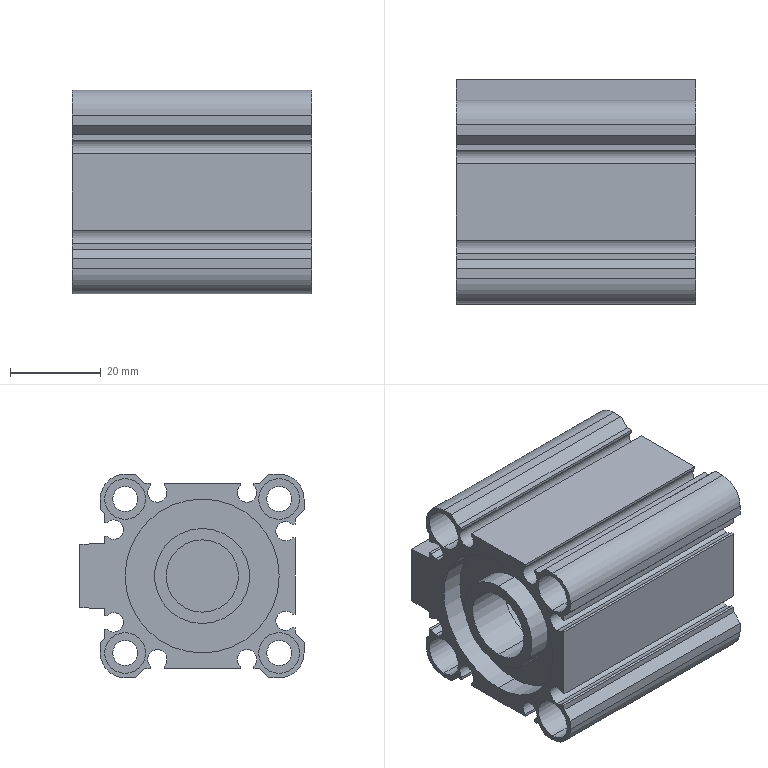Part | SolidWorks | features RefAxis 9, RevCut 5, 3DProfileFeature 3, Extrusion 1, ICE 1, LPattern 1 | 1 solid | 129 faces | box 53 x 49.5 x 45 mm | volume 58938 mm3 | plane 65 | cylinder 60 | cone 4 | commonest cylinder face diameters 4.26 x18 9 x16 5.5 x8 8.566 x4 11 x4 34 x4